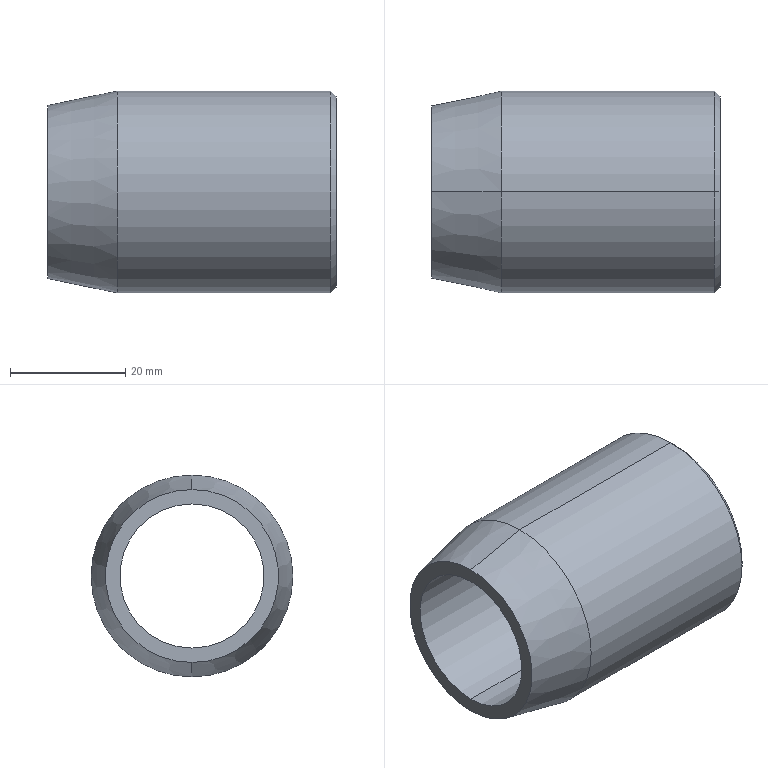Part | SolidWorks | features Chamfer 1, Revolution 1 | 1 solid | 12 faces | box 50 x 35 x 35 mm | volume 21897 mm3 | cone 6 | cylinder 4 | plane 2 | commonest cylinder face diameters 25 x2 35 x2
STEP:
#1=CARTESIAN_POINT('',(0.,0.,-16.5));
#2=VERTEX_POINT('',#1);
#3=CARTESIAN_POINT('',(0.,0.,16.5));
#4=VERTEX_POINT('',#3);
#5=CARTESIAN_POINT('',(0.,0.,0.));
#6=DIRECTION('',(1.,0.,0.));
#7=DIRECTION('',(0.,0.,-1.));
#8=AXIS2_PLACEMENT_3D('',#5,#6,#7);
#9=CIRCLE('',#8,16.5);
#10=EDGE_CURVE('',#2,#4,#9,.T.);
#11=ORIENTED_EDGE('',*,*,#10,.F.);
#12=CARTESIAN_POINT('',(-1.,0.,-17.5));
#13=VERTEX_POINT('',#12);
#14=CARTESIAN_POINT('',(0.,0.,-16.5));
#15=DIRECTION('',(-0.7071,0.,-0.7071));
#16=VECTOR('',#15,1000.);
#17=LINE('',#14,#16);
#18=EDGE_CURVE('',#2,#13,#17,.T.);
#19=ORIENTED_EDGE('',*,*,#18,.T.);
#20=CARTESIAN_POINT('',(-1.,0.,17.5));
#21=VERTEX_POINT('',#20);
#22=CARTESIAN_POINT('',(-1.,0.,0.));
#23=DIRECTION('',(-1.,0.,0.));
#24=DIRECTION('',(0.,0.,-1.));
#25=AXIS2_PLACEMENT_3D('',#22,#23,#24);
#26=CIRCLE('',#25,17.5);
#27=EDGE_CURVE('',#21,#13,#26,.T.);
#28=ORIENTED_EDGE('',*,*,#27,.F.);
#29=CARTESIAN_POINT('',(0.,0.,16.5));
#30=DIRECTION('',(-0.7071,0.,0.7071));
#31=VECTOR('',#30,1000.);
#32=LINE('',#29,#31);
#33=EDGE_CURVE('',#4,#21,#32,.T.);
#34=ORIENTED_EDGE('',*,*,#33,.F.);
#35=EDGE_LOOP('',(#11,#19,#28,#34));
#36=FACE_OUTER_BOUND('',#35,.T.);
#37=CARTESIAN_POINT('',(0.,0.,0.));
#38=DIRECTION('',(-1.,0.,0.));
#39=DIRECTION('',(0.,0.,1.));
#40=AXIS2_PLACEMENT_3D('',#37,#38,#39);
#41=CONICAL_SURFACE('',#40,16.5,0.7854);
#42=ADVANCED_FACE('',(#36),#41,.T.);
#43=CARTESIAN_POINT('',(-1.,0.,12.5));
#44=VERTEX_POINT('',#43);
#45=CARTESIAN_POINT('',(-1.,0.,-12.5));
#46=VERTEX_POINT('',#45);
#47=CARTESIAN_POINT('',(-1.,0.,0.));
#48=DIRECTION('',(1.,0.,0.));
#49=DIRECTION('',(0.,0.,-1.));
#50=AXIS2_PLACEMENT_3D('',#47,#48,#49);
#51=CIRCLE('',#50,12.5);
#52=EDGE_CURVE('',#44,#46,#51,.T.);
#53=ORIENTED_EDGE('',*,*,#52,.F.);
#54=CARTESIAN_POINT('',(0.,0.,13.5));
#55=VERTEX_POINT('',#54);
#56=CARTESIAN_POINT('',(-1.,0.,12.5));
#57=DIRECTION('',(0.7071,0.,0.7071));
#58=VECTOR('',#57,1000.);
#59=LINE('',#56,#58);
#60=EDGE_CURVE('',#44,#55,#59,.T.);
#61=ORIENTED_EDGE('',*,*,#60,.T.);
#62=CARTESIAN_POINT('',(0.,0.,-13.5));
#63=VERTEX_POINT('',#62);
#64=CARTESIAN_POINT('',(0.,0.,0.));
#65=DIRECTION('',(-1.,0.,0.));
#66=DIRECTION('',(0.,0.,-1.));
#67=AXIS2_PLACEMENT_3D('',#64,#65,#66);
#68=CIRCLE('',#67,13.5);
#69=EDGE_CURVE('',#63,#55,#68,.T.);
#70=ORIENTED_EDGE('',*,*,#69,.F.);
#71=CARTESIAN_POINT('',(-1.,0.,-12.5));
#72=DIRECTION('',(0.7071,0.,-0.7071));
#73=VECTOR('',#72,1000.);
#74=LINE('',#71,#73);
#75=EDGE_CURVE('',#46,#63,#74,.T.);
#76=ORIENTED_EDGE('',*,*,#75,.F.);
#77=EDGE_LOOP('',(#53,#61,#70,#76));
#78=FACE_OUTER_BOUND('',#77,.T.);
#79=CARTESIAN_POINT('',(-1.,0.,0.));
#80=DIRECTION('',(1.,0.,0.));
#81=DIRECTION('',(0.,0.,-1.));
#82=AXIS2_PLACEMENT_3D('',#79,#80,#81);
#83=CONICAL_SURFACE('',#82,12.5,0.7854);
#84=ADVANCED_FACE('',(#78),#83,.F.);
#85=CARTESIAN_POINT('',(-50.,0.,-15.));
#86=VERTEX_POINT('',#85);
#87=CARTESIAN_POINT('',(-50.,0.,15.));
#88=VERTEX_POINT('',#87);
#89=CARTESIAN_POINT('',(-50.,0.,0.));
#90=DIRECTION('',(1.,0.,0.));
#91=DIRECTION('',(0.,0.,-1.));
#92=AXIS2_PLACEMENT_3D('',#89,#90,#91);
#93=CIRCLE('',#92,15.);
#94=EDGE_CURVE('',#86,#88,#93,.T.);
#95=ORIENTED_EDGE('',*,*,#94,.T.);
#96=CARTESIAN_POINT('',(-38.,0.,17.5));
#97=VERTEX_POINT('',#96);
#98=CARTESIAN_POINT('',(-38.,0.,17.5));
#99=DIRECTION('',(0.979,0.,0.204));
#100=VECTOR('',#99,1000.);
#101=LINE('',#98,#100);
#102=EDGE_CURVE('',#88,#97,#101,.T.);
#103=ORIENTED_EDGE('',*,*,#102,.T.);
#104=CARTESIAN_POINT('',(-38.,0.,-17.5));
#105=VERTEX_POINT('',#104);
#106=CARTESIAN_POINT('',(-38.,0.,0.));
#107=DIRECTION('',(1.,0.,0.));
#108=DIRECTION('',(0.,0.,-1.));
#109=AXIS2_PLACEMENT_3D('',#106,#107,#108);
#110=CIRCLE('',#109,17.5);
#111=EDGE_CURVE('',#105,#97,#110,.T.);
#112=ORIENTED_EDGE('',*,*,#111,.F.);
#113=CARTESIAN_POINT('',(-38.,0.,-17.5));
#114=DIRECTION('',(0.979,0.,-0.204));
#115=VECTOR('',#114,1000.);
#116=LINE('',#113,#115);
#117=EDGE_CURVE('',#86,#105,#116,.T.);
#118=ORIENTED_EDGE('',*,*,#117,.F.);
#119=EDGE_LOOP('',(#95,#103,#112,#118));
#120=FACE_OUTER_BOUND('',#119,.T.);
#121=CARTESIAN_POINT('',(-38.,0.,0.));
#122=DIRECTION('',(1.,0.,0.));
#123=DIRECTION('',(0.,0.,-1.));
#124=AXIS2_PLACEMENT_3D('',#121,#122,#123);
#125=CONICAL_SURFACE('',#124,17.5,0.2054);
#126=ADVANCED_FACE('',(#120),#125,.T.);
#127=ORIENTED_EDGE('',*,*,#111,.T.);
#128=CARTESIAN_POINT('',(0.,0.,17.5));
#129=DIRECTION('',(1.,0.,0.));
#130=VECTOR('',#129,1000.);
#131=LINE('',#128,#130);
#132=EDGE_CURVE('',#97,#21,#131,.T.);
#133=ORIENTED_EDGE('',*,*,#132,.T.);
#134=ORIENTED_EDGE('',*,*,#27,.T.);
#135=CARTESIAN_POINT('',(0.,0.,-17.5));
#136=DIRECTION('',(1.,0.,0.));
#137=VECTOR('',#136,1000.);
#138=LINE('',#135,#137);
#139=EDGE_CURVE('',#105,#13,#138,.T.);
#140=ORIENTED_EDGE('',*,*,#139,.F.);
#141=EDGE_LOOP('',(#127,#133,#134,#140));
#142=FACE_OUTER_BOUND('',#141,.T.);
#143=CARTESIAN_POINT('',(0.,0.,0.));
#144=DIRECTION('',(1.,0.,0.));
#145=DIRECTION('',(0.,0.,-1.));
#146=AXIS2_PLACEMENT_3D('',#143,#144,#145);
#147=CYLINDRICAL_SURFACE('',#146,17.5);
#148=ADVANCED_FACE('',(#142),#147,.T.);
#149=CARTESIAN_POINT('',(-50.,0.,12.5));
#150=VERTEX_POINT('',#149);
#151=CARTESIAN_POINT('',(-50.,0.,-12.5));
#152=VERTEX_POINT('',#151);
#153=CARTESIAN_POINT('',(-50.,0.,0.));
#154=DIRECTION('',(1.,0.,0.));
#155=DIRECTION('',(0.,0.,-1.));
#156=AXIS2_PLACEMENT_3D('',#153,#154,#155);
#157=CIRCLE('',#156,12.5);
#158=EDGE_CURVE('',#150,#152,#157,.T.);
#159=ORIENTED_EDGE('',*,*,#158,.F.);
#160=CARTESIAN_POINT('',(0.,0.,12.5));
#161=DIRECTION('',(1.,0.,0.));
#162=VECTOR('',#161,1000.);
#163=LINE('',#160,#162);
#164=EDGE_CURVE('',#150,#44,#163,.T.);
#165=ORIENTED_EDGE('',*,*,#164,.T.);
#166=ORIENTED_EDGE('',*,*,#52,.T.);
#167=CARTESIAN_POINT('',(0.,0.,-12.5));
#168=DIRECTION('',(1.,0.,0.));
#169=VECTOR('',#168,1000.);
#170=LINE('',#167,#169);
#171=EDGE_CURVE('',#152,#46,#170,.T.);
#172=ORIENTED_EDGE('',*,*,#171,.F.);
#173=EDGE_LOOP('',(#159,#165,#166,#172));
#174=FACE_OUTER_BOUND('',#173,.T.);
#175=CARTESIAN_POINT('',(0.,0.,0.));
#176=DIRECTION('',(1.,0.,0.));
#177=DIRECTION('',(0.,0.,-1.));
#178=AXIS2_PLACEMENT_3D('',#175,#176,#177);
#179=CYLINDRICAL_SURFACE('',#178,12.5);
#180=ADVANCED_FACE('',(#174),#179,.F.);
#181=ORIENTED_EDGE('',*,*,#164,.F.);
#182=CARTESIAN_POINT('',(-50.,0.,0.));
#183=DIRECTION('',(1.,0.,0.));
#184=DIRECTION('',(0.,0.,-1.));
#185=AXIS2_PLACEMENT_3D('',#182,#183,#184);
#186=CIRCLE('',#185,12.5);
#187=EDGE_CURVE('',#152,#150,#186,.T.);
#188=ORIENTED_EDGE('',*,*,#187,.F.);
#189=ORIENTED_EDGE('',*,*,#171,.T.);
#190=CARTESIAN_POINT('',(-1.,0.,0.));
#191=DIRECTION('',(1.,0.,0.));
#192=DIRECTION('',(0.,0.,-1.));
#193=AXIS2_PLACEMENT_3D('',#190,#191,#192);
#194=CIRCLE('',#193,12.5);
#195=EDGE_CURVE('',#46,#44,#194,.T.);
#196=ORIENTED_EDGE('',*,*,#195,.T.);
#197=EDGE_LOOP('',(#181,#188,#189,#196));
#198=FACE_OUTER_BOUND('',#197,.T.);
#199=CARTESIAN_POINT('',(0.,0.,0.));
#200=DIRECTION('',(1.,0.,0.));
#201=DIRECTION('',(0.,0.,-1.));
#202=AXIS2_PLACEMENT_3D('',#199,#200,#201);
#203=CYLINDRICAL_SURFACE('',#202,12.5);
#204=ADVANCED_FACE('',(#198),#203,.F.);
#205=ORIENTED_EDGE('',*,*,#69,.T.);
#206=CARTESIAN_POINT('',(0.,0.,0.));
#207=DIRECTION('',(-1.,0.,0.));
#208=DIRECTION('',(0.,0.,-1.));
#209=AXIS2_PLACEMENT_3D('',#206,#207,#208);
#210=CIRCLE('',#209,13.5);
#211=EDGE_CURVE('',#55,#63,#210,.T.);
#212=ORIENTED_EDGE('',*,*,#211,.T.);
#213=EDGE_LOOP('',(#205,#212));
#214=FACE_BOUND('',#213,.T.);
#215=CARTESIAN_POINT('',(0.,0.,0.));
#216=DIRECTION('',(1.,0.,0.));
#217=DIRECTION('',(0.,0.,-1.));
#218=AXIS2_PLACEMENT_3D('',#215,#216,#217);
#219=CIRCLE('',#218,16.5);
#220=EDGE_CURVE('',#4,#2,#219,.T.);
#221=ORIENTED_EDGE('',*,*,#220,.T.);
#222=ORIENTED_EDGE('',*,*,#10,.T.);
#223=EDGE_LOOP('',(#221,#222));
#224=FACE_OUTER_BOUND('',#223,.T.);
#225=CARTESIAN_POINT('',(0.,12.5,0.));
#226=DIRECTION('',(1.,0.,0.));
#227=DIRECTION('',(0.,0.,-1.));
#228=AXIS2_PLACEMENT_3D('',#225,#226,#227);
#229=PLANE('',#228);
#230=ADVANCED_FACE('',(#214,#224),#229,.T.);
#231=ORIENTED_EDGE('',*,*,#132,.F.);
#232=CARTESIAN_POINT('',(-38.,0.,0.));
#233=DIRECTION('',(1.,0.,0.));
#234=DIRECTION('',(0.,0.,-1.));
#235=AXIS2_PLACEMENT_3D('',#232,#233,#234);
#236=CIRCLE('',#235,17.5);
#237=EDGE_CURVE('',#97,#105,#236,.T.);
#238=ORIENTED_EDGE('',*,*,#237,.T.);
#239=ORIENTED_EDGE('',*,*,#139,.T.);
#240=CARTESIAN_POINT('',(-1.,0.,0.));
#241=DIRECTION('',(-1.,0.,0.));
#242=DIRECTION('',(0.,0.,-1.));
#243=AXIS2_PLACEMENT_3D('',#240,#241,#242);
#244=CIRCLE('',#243,17.5);
#245=EDGE_CURVE('',#13,#21,#244,.T.);
#246=ORIENTED_EDGE('',*,*,#245,.T.);
#247=EDGE_LOOP('',(#231,#238,#239,#246));
#248=FACE_OUTER_BOUND('',#247,.T.);
#249=CARTESIAN_POINT('',(0.,0.,0.));
#250=DIRECTION('',(1.,0.,0.));
#251=DIRECTION('',(0.,0.,-1.));
#252=AXIS2_PLACEMENT_3D('',#249,#250,#251);
#253=CYLINDRICAL_SURFACE('',#252,17.5);
#254=ADVANCED_FACE('',(#248),#253,.T.);
#255=ORIENTED_EDGE('',*,*,#102,.F.);
#256=CARTESIAN_POINT('',(-50.,0.,0.));
#257=DIRECTION('',(1.,0.,0.));
#258=DIRECTION('',(0.,0.,-1.));
#259=AXIS2_PLACEMENT_3D('',#256,#257,#258);
#260=CIRCLE('',#259,15.);
#261=EDGE_CURVE('',#88,#86,#260,.T.);
#262=ORIENTED_EDGE('',*,*,#261,.T.);
#263=ORIENTED_EDGE('',*,*,#117,.T.);
#264=ORIENTED_EDGE('',*,*,#237,.F.);
#265=EDGE_LOOP('',(#255,#262,#263,#264));
#266=FACE_OUTER_BOUND('',#265,.T.);
#267=CARTESIAN_POINT('',(-38.,0.,0.));
#268=DIRECTION('',(1.,0.,0.));
#269=DIRECTION('',(0.,0.,-1.));
#270=AXIS2_PLACEMENT_3D('',#267,#268,#269);
#271=CONICAL_SURFACE('',#270,17.5,0.2054);
#272=ADVANCED_FACE('',(#266),#271,.T.);
#273=ORIENTED_EDGE('',*,*,#187,.T.);
#274=ORIENTED_EDGE('',*,*,#158,.T.);
#275=EDGE_LOOP('',(#273,#274));
#276=FACE_BOUND('',#275,.T.);
#277=ORIENTED_EDGE('',*,*,#94,.F.);
#278=ORIENTED_EDGE('',*,*,#261,.F.);
#279=EDGE_LOOP('',(#277,#278));
#280=FACE_OUTER_BOUND('',#279,.T.);
#281=CARTESIAN_POINT('',(-50.,15.,0.));
#282=DIRECTION('',(-1.,0.,0.));
#283=DIRECTION('',(0.,0.,1.));
#284=AXIS2_PLACEMENT_3D('',#281,#282,#283);
#285=PLANE('',#284);
#286=ADVANCED_FACE('',(#276,#280),#285,.T.);
#287=ORIENTED_EDGE('',*,*,#60,.F.);
#288=ORIENTED_EDGE('',*,*,#195,.F.);
#289=ORIENTED_EDGE('',*,*,#75,.T.);
#290=ORIENTED_EDGE('',*,*,#211,.F.);
#291=EDGE_LOOP('',(#287,#288,#289,#290));
#292=FACE_OUTER_BOUND('',#291,.T.);
#293=CARTESIAN_POINT('',(-1.,0.,0.));
#294=DIRECTION('',(1.,0.,0.));
#295=DIRECTION('',(0.,0.,-1.));
#296=AXIS2_PLACEMENT_3D('',#293,#294,#295);
#297=CONICAL_SURFACE('',#296,12.5,0.7854);
#298=ADVANCED_FACE('',(#292),#297,.F.);
#299=ORIENTED_EDGE('',*,*,#18,.F.);
#300=ORIENTED_EDGE('',*,*,#220,.F.);
#301=ORIENTED_EDGE('',*,*,#33,.T.);
#302=ORIENTED_EDGE('',*,*,#245,.F.);
#303=EDGE_LOOP('',(#299,#300,#301,#302));
#304=FACE_OUTER_BOUND('',#303,.T.);
#305=CARTESIAN_POINT('',(0.,0.,0.));
#306=DIRECTION('',(-1.,0.,0.));
#307=DIRECTION('',(0.,0.,1.));
#308=AXIS2_PLACEMENT_3D('',#305,#306,#307);
#309=CONICAL_SURFACE('',#308,16.5,0.7854);
#310=ADVANCED_FACE('',(#304),#309,.T.);
#311=CLOSED_SHELL('',(#42,#84,#126,#148,#180,#204,#230,#254,#272,#286,#298,#310));
#312=MANIFOLD_SOLID_BREP('',#311);
#313=CARTESIAN_POINT('',(0.,0.,0.));
#314=DIRECTION('',(0.,0.,1.));
#315=DIRECTION('',(1.,0.,0.));
#316=AXIS2_PLACEMENT_3D('',#313,#314,#315);
#317=(LENGTH_UNIT()NAMED_UNIT(*)SI_UNIT(.MILLI.,.METRE.));
#318=UNCERTAINTY_MEASURE_WITH_UNIT(LENGTH_MEASURE(0.00001),#317,'','');
#319=(NAMED_UNIT(*)PLANE_ANGLE_UNIT()SI_UNIT($,.RADIAN.));
#320=(NAMED_UNIT(*)SI_UNIT($,.STERADIAN.)SOLID_ANGLE_UNIT());
#321=(GEOMETRIC_REPRESENTATION_CONTEXT(3)GLOBAL_UNCERTAINTY_ASSIGNED_CONTEXT((#318))GLOBAL_UNIT_ASSIGNED_CONTEXT((#317,#319,#320))REPRESENTATION_CONTEXT('',''));
#322=ADVANCED_BREP_SHAPE_REPRESENTATION('',(#312,#316),#321);